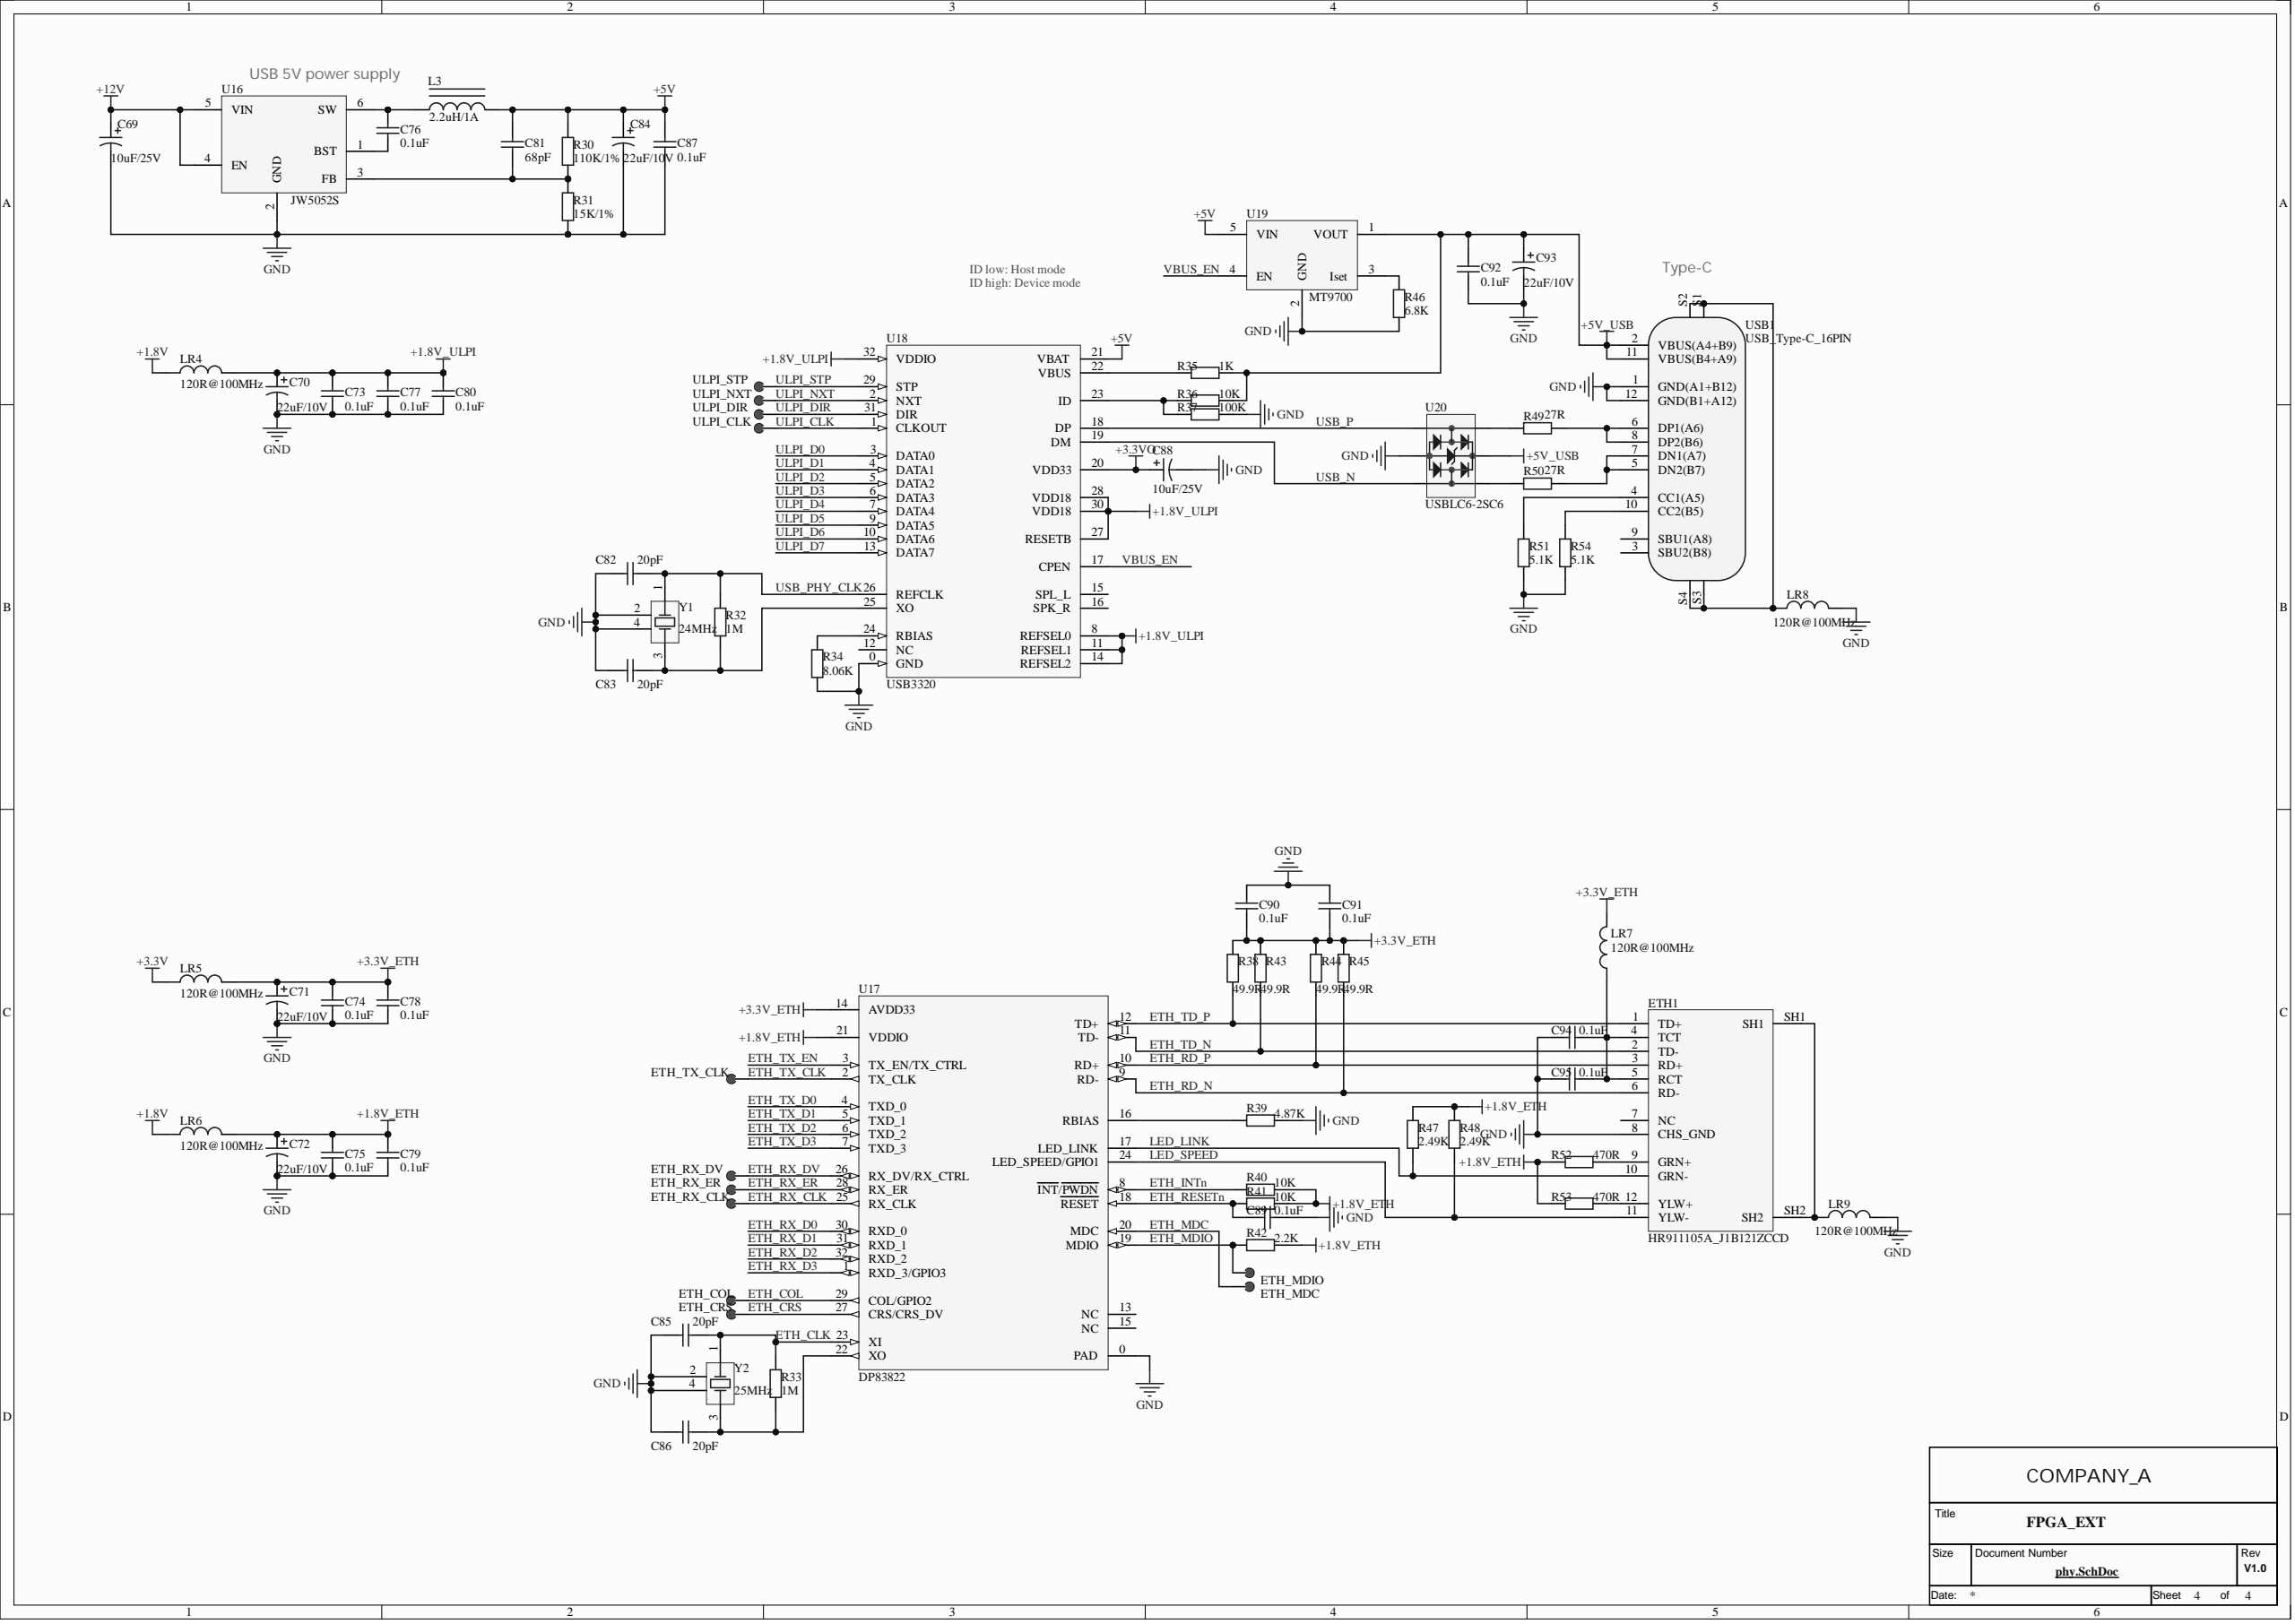Circuit board | Altium Designer | 234 parts | 308 nets | one sheet of the schematic
Parts on this sheet (reference | value | footprint):
C69 | 10uF/25V | 0603C_N
C70 | 22uF/10V | 0603C_N
C71 | 22uF/10V | 0603C_N
C72 | 22uF/10V | 0603C_N
C73 | 0.1uF | 0603C_N
C74 | 0.1uF | 0603C_N
C75 | 0.1uF | 0603C_N
C76 | 0.1uF | 0603C_N
C77 | 0.1uF | 0603C_N
C78 | 0.1uF | 0603C_N
C79 | 0.1uF | 0603C_N
C80 | 0.1uF | 0603C_N
C81 | 68pF | 0603C_N
C82 | 20pF | 0603C_N
C83 | 20pF | 0603C_N
C84 | 22uF/10V | 0603C_N
C85 | 20pF | 0603C_N
C86 | 20pF | 0603C_N
C87 | 0.1uF | 0603C_N
C88 | 10uF/25V | 0603C_N
C89 | 0.1uF | 0603C_N
C90 | 0.1uF | 0603C_N
C91 | 0.1uF | 0603C_N
C92 | 0.1uF | 0603C_N
C93 | 22uF/10V | 0603C_N
C94 | 0.1uF | 0603C_N
C95 | 0.1uF | 0603C_N
ETH1 | HR911105A_J1B121ZCCD | RJ45_HR911003A
L3 | 2.2uH/1A | LD-5.5mm
LR4 | 120R@100MHz | 0603R_N
LR5 | 120R@100MHz | 0603R_N
LR6 | 120R@100MHz | 0603R_N
LR7 | 120R@100MHz | 0603R_N
LR8 | 120R@100MHz | 0603R_N
LR9 | 120R@100MHz | 0603R_N
R30 | 110K/1% | 0603R_N
R31 | 15K/1% | 0603R_N
R32 | 1M | 0603R_N
R33 | 1M | 0603R_N
R34 | 8.06K | 0603R_N
R35 | 1K | 0603R_N
R36 | 10K | 0603R_N
R37 | 100K | 0603R_N
R38 | 49.9R | 0603R_N
R39 | 4.87K | 0603R_N
R40 | 10K | 0603R_N
R41 | 10K | 0603R_N
R42 | 2.2K | 0603R_N
R43 | 49.9R | 0603R_N
R44 | 49.9R | 0603R_N
R45 | 49.9R | 0603R_N
R46 | 6.8K | 0603R_N
R47 | 2.49K | 0603R_N
R48 | 2.49K | 0603R_N
R51 | 5.1K | 0603R_N
R52 | 470R | 0603R_N
R53 | 470R | 0603R_N
R54 | 5.1K | 0603R_N
U16 | JW5052S | SOT-23-6
U17 | DP83822 | QFN32 5X5
U18 | USB3320 | QFN32 5x5
U19 | MT9700 | SOT-23-5
U20 | USBLC6-2SC6 | SOT-23-6
USB1 | USB_Type-C_16PIN | USB_Type-C_16PIN
Y1 | 24MHz | XTAL_SMD3225
Y2 | 25MHz | XTAL_SMD3225
Nets of these parts (net: part-pin ...):
VBUS_EN: U19-4 U18-17
USB_PHY_CLK: C82-1 R32-2 Y1-1 U18-26
USB_P: U20-3 U18-18
USB_N: U20-1 U18-19
ULPI_STP: U18-29
ULPI_NXT: U18-2
ULPI_DIR: U18-31
ULPI_D7: U18-13
ULPI_D6: U18-10
ULPI_D5: U18-9
ULPI_D4: U18-7
ULPI_D3: U18-6
ULPI_D2: U18-5
ULPI_D1: U18-4
ULPI_D0: U18-3
ULPI_CLK: U18-1
NetR54_2: R54-2 USB1-10
NetR51_2: R51-2 USB1-4
NetR50_2: USB1-5 USB1-7
NetR50_1: U20-6
NetR49_2: USB1-6 USB1-8
NetR49_1: U20-4
NetR46_2: R46-2 U19-3
NetR39_2: R39-2 U17-16
NetR36_1: R36-1 R37-1 U18-23
NetR35_1: R35-1 U18-22
NetR34_1: R34-1 U18-24
NetLR8_2: LR8-2 USB1-S1 USB1-S2 USB1-S3 USB1-S4
NetETH1_SH1: ETH1-SH1 ETH1-SH2 LR9-2
NetETH1_12: ETH1-12 R53-2
NetETH1_9: ETH1-9 R52-2
NetC94_2: C94-2 C95-2 ETH1-4 ETH1-5 LR7-2
NetC86_1: C86-1 R33-1 Y2-3 U17-22
NetC83_1: C83-1 R32-1 Y1-3 U18-25
NetC81_2: C81-2 R30-2 R31-1 U16-3
NetC76_2: C76-2 L3-1 U16-6
NetC76_1: C76-1 U16-1
LED_SPEED: ETH1-11 R48-2 U17-24
LED_LINK: ETH1-10 R47-2 U17-17
GND: C69-2 C70-2 C71-2 C72-2 C73-1 C74-1 C75-1 C77-1 C78-1 C79-1 C80-2 C82-2 C83-2 C84-2 C85-2 C86-2 C87-1 C88-2 C89-1 C90-1 C91-1 C92-2 C93-2 C94-1 C95-1 ETH1-8 LR8-1 LR9-1 R31-2 R34-2 R37-2 R39-1 R46-1 R51-1 R54-1 U16-2 U19-2 U20-2 USB1-1 USB1-12 Y1-2 Y1-4 Y2-2 Y2-4 U17-0 U18-0
ETH_TX_EN: U17-3
ETH_TX_D3: U17-7
ETH_TX_D2: U17-6
ETH_TX_D1: U17-5
ETH_TX_D0: U17-4
ETH_TX_CLK: U17-2
ETH_TD_P: ETH1-1 R38-1 U17-12
ETH_TD_N: ETH1-2 R43-1 U17-11
ETH_RX_ER: U17-28
ETH_RX_DV: U17-26
ETH_RX_D3: U17-1
ETH_RX_D2: U17-32
ETH_RX_D1: U17-31
ETH_RX_D0: U17-30
ETH_RX_CLK: U17-25
ETH_RESETn: C89-2 R41-2 U17-18
ETH_RD_P: ETH1-3 R44-1 U17-10
ETH_RD_N: ETH1-6 R45-1 U17-9
ETH_MDIO: R42-2 U17-19
ETH_MDC: U17-20
ETH_INTn: R40-2 U17-8
ETH_CRS: U17-27
ETH_COL: U17-29
ETH_CLK: C85-1 R33-2 Y2-1 U17-23
+12V: C69-1 U16-4 U16-5
+5V_USB: C92-1 C93-1 R35-2 R36-2 U19-1 U20-5 USB1-2 USB1-11
+5V: C81-1 C84-1 C87-2 L3-2 R30-1 U19-5 U18-21
+3.3VO: C88-1 U18-20
+3.3V_ETH: C71-1 C74-2 C78-2 C90-2 C91-2 LR5-1 LR7-1 R38-2 R43-2 R44-2 R45-2 U17-14
+3.3V: LR5-2
+1.8V_ULPI: C70-1 C73-2 C77-2 C80-1 LR4-1 U18-8 U18-11 U18-14 U18-27 U18-28 U18-30 U18-32
+1.8V_ETH: C72-1 C75-2 C79-2 LR6-1 R40-1 R41-1 R42-1 R47-1 R48-1 R52-1 R53-1 U17-21
+1.8V: LR4-2 LR6-2